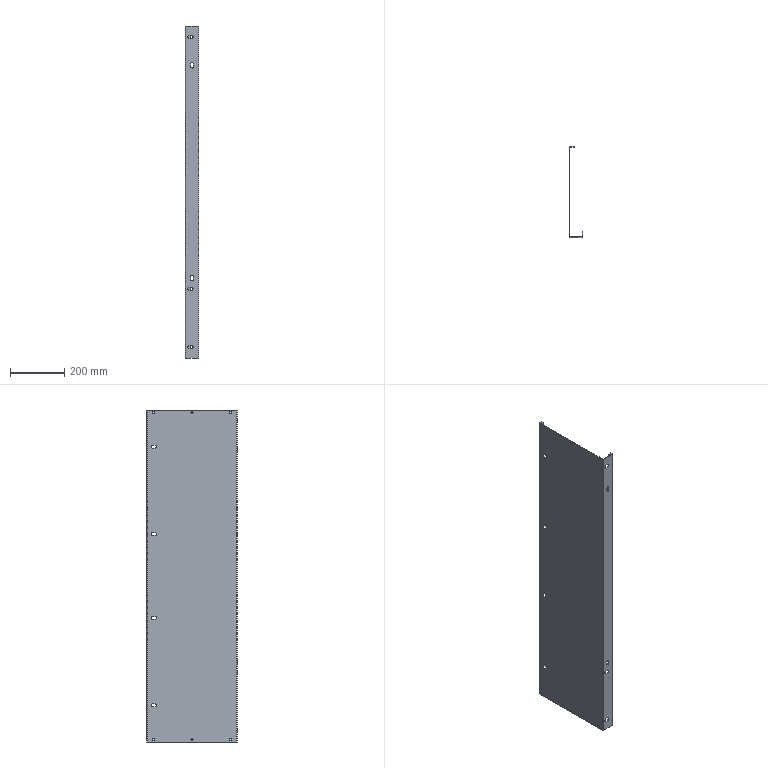Part | SolidWorks | features ICE 8, Cut 4, Chamfer 1, FlatPattern 1, SMBaseFlange 1, SheetMetal 1 | 1 solid | 88 faces | box 50 x 333 x 1221 mm | volume 608956 mm3 | plane 46 | cylinder 42 | commonest cylinder face diameters 10 x24 8 x12 2 x3 4.4 x3